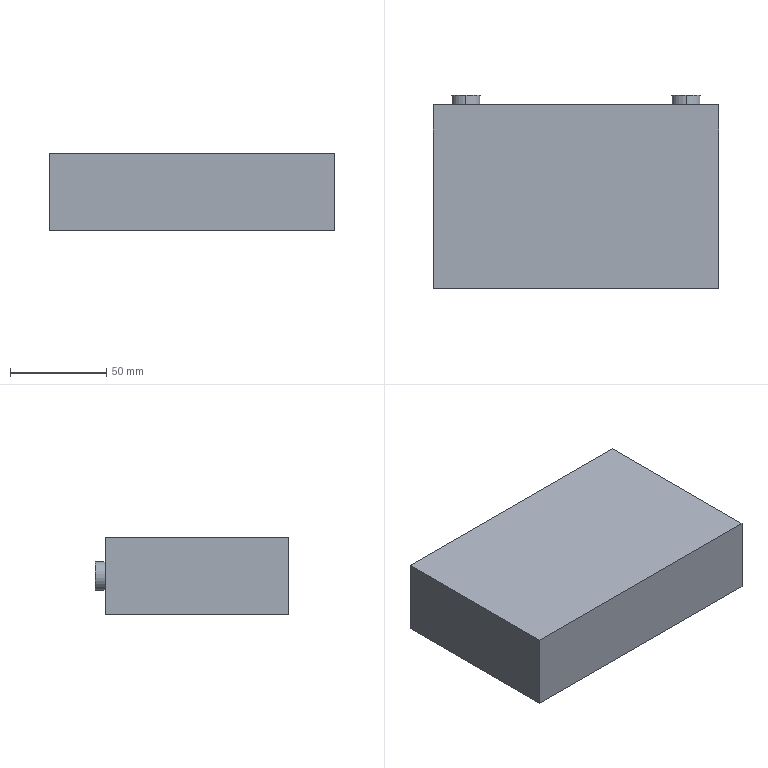Part | SolidWorks | features Extrusion 1, ICE 1 | 1 solid | 12 faces | box 148.9 x 100.6 x 40.2 mm | volume 574008 mm3 | plane 8 | cylinder 4 | commonest cylinder face diameters 15 x4
STEP:
#1=CARTESIAN_POINT('',(-57.3,100.6,7.5));
#2=VERTEX_POINT('',#1);
#3=CARTESIAN_POINT('',(-57.3,100.6,-7.5));
#4=VERTEX_POINT('',#3);
#5=CARTESIAN_POINT('',(-57.3,100.6,0.));
#6=DIRECTION('',(0.,1.,0.));
#7=DIRECTION('',(0.,0.,1.));
#8=AXIS2_PLACEMENT_3D('',#5,#6,#7);
#9=CIRCLE('',#8,7.5);
#10=EDGE_CURVE('',#2,#4,#9,.T.);
#11=ORIENTED_EDGE('',*,*,#10,.F.);
#12=CARTESIAN_POINT('',(-57.3,95.6,7.5));
#13=VERTEX_POINT('',#12);
#14=CARTESIAN_POINT('',(-57.3,100.6,7.5));
#15=DIRECTION('',(0.,-1.,0.));
#16=VECTOR('',#15,1000.);
#17=LINE('',#14,#16);
#18=EDGE_CURVE('',#2,#13,#17,.T.);
#19=ORIENTED_EDGE('',*,*,#18,.T.);
#20=CARTESIAN_POINT('',(-57.3,95.6,-7.5));
#21=VERTEX_POINT('',#20);
#22=CARTESIAN_POINT('',(-57.3,95.6,0.));
#23=DIRECTION('',(0.,1.,0.));
#24=DIRECTION('',(0.,0.,1.));
#25=AXIS2_PLACEMENT_3D('',#22,#23,#24);
#26=CIRCLE('',#25,7.5);
#27=EDGE_CURVE('',#13,#21,#26,.T.);
#28=ORIENTED_EDGE('',*,*,#27,.T.);
#29=CARTESIAN_POINT('',(-57.3,100.6,-7.5));
#30=DIRECTION('',(0.,-1.,0.));
#31=VECTOR('',#30,1000.);
#32=LINE('',#29,#31);
#33=EDGE_CURVE('',#4,#21,#32,.T.);
#34=ORIENTED_EDGE('',*,*,#33,.F.);
#35=EDGE_LOOP('',(#11,#19,#28,#34));
#36=FACE_OUTER_BOUND('',#35,.T.);
#37=CARTESIAN_POINT('',(-57.3,100.6,0.));
#38=DIRECTION('',(0.,-1.,0.));
#39=DIRECTION('',(0.,0.,-1.));
#40=AXIS2_PLACEMENT_3D('',#37,#38,#39);
#41=CYLINDRICAL_SURFACE('',#40,7.5);
#42=ADVANCED_FACE('',(#36),#41,.T.);
#43=CARTESIAN_POINT('',(57.3,100.6,7.5));
#44=VERTEX_POINT('',#43);
#45=CARTESIAN_POINT('',(57.3,100.6,-7.5));
#46=VERTEX_POINT('',#45);
#47=CARTESIAN_POINT('',(57.3,100.6,0.));
#48=DIRECTION('',(0.,1.,0.));
#49=DIRECTION('',(0.,0.,1.));
#50=AXIS2_PLACEMENT_3D('',#47,#48,#49);
#51=CIRCLE('',#50,7.5);
#52=EDGE_CURVE('',#44,#46,#51,.T.);
#53=ORIENTED_EDGE('',*,*,#52,.F.);
#54=CARTESIAN_POINT('',(57.3,95.6,7.5));
#55=VERTEX_POINT('',#54);
#56=CARTESIAN_POINT('',(57.3,100.6,7.5));
#57=DIRECTION('',(0.,-1.,0.));
#58=VECTOR('',#57,1000.);
#59=LINE('',#56,#58);
#60=EDGE_CURVE('',#44,#55,#59,.T.);
#61=ORIENTED_EDGE('',*,*,#60,.T.);
#62=CARTESIAN_POINT('',(57.3,95.6,-7.5));
#63=VERTEX_POINT('',#62);
#64=CARTESIAN_POINT('',(57.3,95.6,0.));
#65=DIRECTION('',(0.,1.,0.));
#66=DIRECTION('',(0.,0.,1.));
#67=AXIS2_PLACEMENT_3D('',#64,#65,#66);
#68=CIRCLE('',#67,7.5);
#69=EDGE_CURVE('',#55,#63,#68,.T.);
#70=ORIENTED_EDGE('',*,*,#69,.T.);
#71=CARTESIAN_POINT('',(57.3,100.6,-7.5));
#72=DIRECTION('',(0.,-1.,0.));
#73=VECTOR('',#72,1000.);
#74=LINE('',#71,#73);
#75=EDGE_CURVE('',#46,#63,#74,.T.);
#76=ORIENTED_EDGE('',*,*,#75,.F.);
#77=EDGE_LOOP('',(#53,#61,#70,#76));
#78=FACE_OUTER_BOUND('',#77,.T.);
#79=CARTESIAN_POINT('',(57.3,100.6,0.));
#80=DIRECTION('',(0.,-1.,0.));
#81=DIRECTION('',(0.,0.,-1.));
#82=AXIS2_PLACEMENT_3D('',#79,#80,#81);
#83=CYLINDRICAL_SURFACE('',#82,7.5);
#84=ADVANCED_FACE('',(#78),#83,.T.);
#85=CARTESIAN_POINT('',(57.3,95.6,0.));
#86=DIRECTION('',(0.,1.,0.));
#87=DIRECTION('',(0.,0.,1.));
#88=AXIS2_PLACEMENT_3D('',#85,#86,#87);
#89=CIRCLE('',#88,7.5);
#90=EDGE_CURVE('',#63,#55,#89,.T.);
#91=ORIENTED_EDGE('',*,*,#90,.F.);
#92=ORIENTED_EDGE('',*,*,#69,.F.);
#93=EDGE_LOOP('',(#91,#92));
#94=FACE_BOUND('',#93,.T.);
#95=CARTESIAN_POINT('',(74.45,95.6,20.1));
#96=VERTEX_POINT('',#95);
#97=CARTESIAN_POINT('',(74.45,95.6,-20.1));
#98=VERTEX_POINT('',#97);
#99=CARTESIAN_POINT('',(74.45,95.6,-20.1));
#100=DIRECTION('',(0.,0.,-1.));
#101=VECTOR('',#100,1000.);
#102=LINE('',#99,#101);
#103=EDGE_CURVE('',#96,#98,#102,.T.);
#104=ORIENTED_EDGE('',*,*,#103,.T.);
#105=CARTESIAN_POINT('',(-74.45,95.6,-20.1));
#106=VERTEX_POINT('',#105);
#107=CARTESIAN_POINT('',(-74.45,95.6,-20.1));
#108=DIRECTION('',(-1.,0.,0.));
#109=VECTOR('',#108,1000.);
#110=LINE('',#107,#109);
#111=EDGE_CURVE('',#98,#106,#110,.T.);
#112=ORIENTED_EDGE('',*,*,#111,.T.);
#113=CARTESIAN_POINT('',(-74.45,95.6,20.1));
#114=VERTEX_POINT('',#113);
#115=CARTESIAN_POINT('',(-74.45,95.6,-20.1));
#116=DIRECTION('',(0.,0.,1.));
#117=VECTOR('',#116,1000.);
#118=LINE('',#115,#117);
#119=EDGE_CURVE('',#106,#114,#118,.T.);
#120=ORIENTED_EDGE('',*,*,#119,.T.);
#121=CARTESIAN_POINT('',(-74.45,95.6,20.1));
#122=DIRECTION('',(1.,0.,0.));
#123=VECTOR('',#122,1000.);
#124=LINE('',#121,#123);
#125=EDGE_CURVE('',#114,#96,#124,.T.);
#126=ORIENTED_EDGE('',*,*,#125,.T.);
#127=EDGE_LOOP('',(#104,#112,#120,#126));
#128=FACE_OUTER_BOUND('',#127,.T.);
#129=CARTESIAN_POINT('',(-57.3,95.6,0.));
#130=DIRECTION('',(0.,1.,0.));
#131=DIRECTION('',(0.,0.,1.));
#132=AXIS2_PLACEMENT_3D('',#129,#130,#131);
#133=CIRCLE('',#132,7.5);
#134=EDGE_CURVE('',#21,#13,#133,.T.);
#135=ORIENTED_EDGE('',*,*,#134,.F.);
#136=ORIENTED_EDGE('',*,*,#27,.F.);
#137=EDGE_LOOP('',(#135,#136));
#138=FACE_BOUND('',#137,.T.);
#139=CARTESIAN_POINT('',(0.,95.6,0.));
#140=DIRECTION('',(0.,1.,0.));
#141=DIRECTION('',(0.,0.,1.));
#142=AXIS2_PLACEMENT_3D('',#139,#140,#141);
#143=PLANE('',#142);
#144=ADVANCED_FACE('',(#94,#128,#138),#143,.T.);
#145=CARTESIAN_POINT('',(74.45,0.,20.1));
#146=VERTEX_POINT('',#145);
#147=CARTESIAN_POINT('',(74.45,0.,-20.1));
#148=VERTEX_POINT('',#147);
#149=CARTESIAN_POINT('',(74.45,0.,-20.1));
#150=DIRECTION('',(0.,0.,-1.));
#151=VECTOR('',#150,1000.);
#152=LINE('',#149,#151);
#153=EDGE_CURVE('',#146,#148,#152,.T.);
#154=ORIENTED_EDGE('',*,*,#153,.T.);
#155=CARTESIAN_POINT('',(74.45,95.6,-20.1));
#156=DIRECTION('',(0.,-1.,0.));
#157=VECTOR('',#156,1000.);
#158=LINE('',#155,#157);
#159=EDGE_CURVE('',#98,#148,#158,.T.);
#160=ORIENTED_EDGE('',*,*,#159,.F.);
#161=ORIENTED_EDGE('',*,*,#103,.F.);
#162=CARTESIAN_POINT('',(74.45,95.6,20.1));
#163=DIRECTION('',(0.,-1.,0.));
#164=VECTOR('',#163,1000.);
#165=LINE('',#162,#164);
#166=EDGE_CURVE('',#96,#146,#165,.T.);
#167=ORIENTED_EDGE('',*,*,#166,.T.);
#168=EDGE_LOOP('',(#154,#160,#161,#167));
#169=FACE_OUTER_BOUND('',#168,.T.);
#170=CARTESIAN_POINT('',(74.45,95.6,-20.1));
#171=DIRECTION('',(-1.,0.,0.));
#172=DIRECTION('',(0.,0.,1.));
#173=AXIS2_PLACEMENT_3D('',#170,#171,#172);
#174=PLANE('',#173);
#175=ADVANCED_FACE('',(#169),#174,.F.);
#176=CARTESIAN_POINT('',(-74.45,0.,-20.1));
#177=VERTEX_POINT('',#176);
#178=CARTESIAN_POINT('',(-74.45,0.,-20.1));
#179=DIRECTION('',(-1.,0.,0.));
#180=VECTOR('',#179,1000.);
#181=LINE('',#178,#180);
#182=EDGE_CURVE('',#148,#177,#181,.T.);
#183=ORIENTED_EDGE('',*,*,#182,.T.);
#184=CARTESIAN_POINT('',(-74.45,95.6,-20.1));
#185=DIRECTION('',(0.,-1.,0.));
#186=VECTOR('',#185,1000.);
#187=LINE('',#184,#186);
#188=EDGE_CURVE('',#106,#177,#187,.T.);
#189=ORIENTED_EDGE('',*,*,#188,.F.);
#190=ORIENTED_EDGE('',*,*,#111,.F.);
#191=ORIENTED_EDGE('',*,*,#159,.T.);
#192=EDGE_LOOP('',(#183,#189,#190,#191));
#193=FACE_OUTER_BOUND('',#192,.T.);
#194=CARTESIAN_POINT('',(-74.45,95.6,-20.1));
#195=DIRECTION('',(0.,0.,1.));
#196=DIRECTION('',(1.,0.,0.));
#197=AXIS2_PLACEMENT_3D('',#194,#195,#196);
#198=PLANE('',#197);
#199=ADVANCED_FACE('',(#193),#198,.F.);
#200=CARTESIAN_POINT('',(-74.45,0.,20.1));
#201=VERTEX_POINT('',#200);
#202=CARTESIAN_POINT('',(-74.45,0.,-20.1));
#203=DIRECTION('',(0.,0.,1.));
#204=VECTOR('',#203,1000.);
#205=LINE('',#202,#204);
#206=EDGE_CURVE('',#177,#201,#205,.T.);
#207=ORIENTED_EDGE('',*,*,#206,.T.);
#208=CARTESIAN_POINT('',(-74.45,95.6,20.1));
#209=DIRECTION('',(0.,-1.,0.));
#210=VECTOR('',#209,1000.);
#211=LINE('',#208,#210);
#212=EDGE_CURVE('',#114,#201,#211,.T.);
#213=ORIENTED_EDGE('',*,*,#212,.F.);
#214=ORIENTED_EDGE('',*,*,#119,.F.);
#215=ORIENTED_EDGE('',*,*,#188,.T.);
#216=EDGE_LOOP('',(#207,#213,#214,#215));
#217=FACE_OUTER_BOUND('',#216,.T.);
#218=CARTESIAN_POINT('',(-74.45,95.6,-20.1));
#219=DIRECTION('',(1.,0.,0.));
#220=DIRECTION('',(0.,0.,-1.));
#221=AXIS2_PLACEMENT_3D('',#218,#219,#220);
#222=PLANE('',#221);
#223=ADVANCED_FACE('',(#217),#222,.F.);
#224=CARTESIAN_POINT('',(-74.45,0.,20.1));
#225=DIRECTION('',(1.,0.,0.));
#226=VECTOR('',#225,1000.);
#227=LINE('',#224,#226);
#228=EDGE_CURVE('',#201,#146,#227,.T.);
#229=ORIENTED_EDGE('',*,*,#228,.T.);
#230=ORIENTED_EDGE('',*,*,#166,.F.);
#231=ORIENTED_EDGE('',*,*,#125,.F.);
#232=ORIENTED_EDGE('',*,*,#212,.T.);
#233=EDGE_LOOP('',(#229,#230,#231,#232));
#234=FACE_OUTER_BOUND('',#233,.T.);
#235=CARTESIAN_POINT('',(-74.45,95.6,20.1));
#236=DIRECTION('',(0.,0.,-1.));
#237=DIRECTION('',(-1.,0.,0.));
#238=AXIS2_PLACEMENT_3D('',#235,#236,#237);
#239=PLANE('',#238);
#240=ADVANCED_FACE('',(#234),#239,.F.);
#241=ORIENTED_EDGE('',*,*,#153,.F.);
#242=ORIENTED_EDGE('',*,*,#228,.F.);
#243=ORIENTED_EDGE('',*,*,#206,.F.);
#244=ORIENTED_EDGE('',*,*,#182,.F.);
#245=EDGE_LOOP('',(#241,#242,#243,#244));
#246=FACE_OUTER_BOUND('',#245,.T.);
#247=CARTESIAN_POINT('',(0.,0.,0.));
#248=DIRECTION('',(0.,1.,0.));
#249=DIRECTION('',(0.,0.,1.));
#250=AXIS2_PLACEMENT_3D('',#247,#248,#249);
#251=PLANE('',#250);
#252=ADVANCED_FACE('',(#246),#251,.F.);
#253=ORIENTED_EDGE('',*,*,#60,.F.);
#254=CARTESIAN_POINT('',(57.3,100.6,0.));
#255=DIRECTION('',(0.,1.,0.));
#256=DIRECTION('',(0.,0.,1.));
#257=AXIS2_PLACEMENT_3D('',#254,#255,#256);
#258=CIRCLE('',#257,7.5);
#259=EDGE_CURVE('',#46,#44,#258,.T.);
#260=ORIENTED_EDGE('',*,*,#259,.F.);
#261=ORIENTED_EDGE('',*,*,#75,.T.);
#262=ORIENTED_EDGE('',*,*,#90,.T.);
#263=EDGE_LOOP('',(#253,#260,#261,#262));
#264=FACE_OUTER_BOUND('',#263,.T.);
#265=CARTESIAN_POINT('',(57.3,100.6,0.));
#266=DIRECTION('',(0.,-1.,0.));
#267=DIRECTION('',(0.,0.,-1.));
#268=AXIS2_PLACEMENT_3D('',#265,#266,#267);
#269=CYLINDRICAL_SURFACE('',#268,7.5);
#270=ADVANCED_FACE('',(#264),#269,.T.);
#271=ORIENTED_EDGE('',*,*,#259,.T.);
#272=ORIENTED_EDGE('',*,*,#52,.T.);
#273=EDGE_LOOP('',(#271,#272));
#274=FACE_OUTER_BOUND('',#273,.T.);
#275=CARTESIAN_POINT('',(57.3,100.6,0.));
#276=DIRECTION('',(0.,1.,0.));
#277=DIRECTION('',(0.,0.,1.));
#278=AXIS2_PLACEMENT_3D('',#275,#276,#277);
#279=PLANE('',#278);
#280=ADVANCED_FACE('',(#274),#279,.T.);
#281=ORIENTED_EDGE('',*,*,#18,.F.);
#282=CARTESIAN_POINT('',(-57.3,100.6,0.));
#283=DIRECTION('',(0.,1.,0.));
#284=DIRECTION('',(0.,0.,1.));
#285=AXIS2_PLACEMENT_3D('',#282,#283,#284);
#286=CIRCLE('',#285,7.5);
#287=EDGE_CURVE('',#4,#2,#286,.T.);
#288=ORIENTED_EDGE('',*,*,#287,.F.);
#289=ORIENTED_EDGE('',*,*,#33,.T.);
#290=ORIENTED_EDGE('',*,*,#134,.T.);
#291=EDGE_LOOP('',(#281,#288,#289,#290));
#292=FACE_OUTER_BOUND('',#291,.T.);
#293=CARTESIAN_POINT('',(-57.3,100.6,0.));
#294=DIRECTION('',(0.,-1.,0.));
#295=DIRECTION('',(0.,0.,-1.));
#296=AXIS2_PLACEMENT_3D('',#293,#294,#295);
#297=CYLINDRICAL_SURFACE('',#296,7.5);
#298=ADVANCED_FACE('',(#292),#297,.T.);
#299=ORIENTED_EDGE('',*,*,#287,.T.);
#300=ORIENTED_EDGE('',*,*,#10,.T.);
#301=EDGE_LOOP('',(#299,#300));
#302=FACE_OUTER_BOUND('',#301,.T.);
#303=CARTESIAN_POINT('',(-57.3,100.6,0.));
#304=DIRECTION('',(0.,1.,0.));
#305=DIRECTION('',(0.,0.,1.));
#306=AXIS2_PLACEMENT_3D('',#303,#304,#305);
#307=PLANE('',#306);
#308=ADVANCED_FACE('',(#302),#307,.T.);
#309=CLOSED_SHELL('',(#42,#84,#144,#175,#199,#223,#240,#252,#270,#280,#298,#308));
#310=MANIFOLD_SOLID_BREP('',#309);
#311=CARTESIAN_POINT('',(0.,0.,0.));
#312=DIRECTION('',(0.,0.,1.));
#313=DIRECTION('',(1.,0.,0.));
#314=AXIS2_PLACEMENT_3D('',#311,#312,#313);
#315=(LENGTH_UNIT()NAMED_UNIT(*)SI_UNIT(.MILLI.,.METRE.));
#316=UNCERTAINTY_MEASURE_WITH_UNIT(LENGTH_MEASURE(0.00001),#315,'','');
#317=(NAMED_UNIT(*)PLANE_ANGLE_UNIT()SI_UNIT($,.RADIAN.));
#318=(NAMED_UNIT(*)SI_UNIT($,.STERADIAN.)SOLID_ANGLE_UNIT());
#319=(GEOMETRIC_REPRESENTATION_CONTEXT(3)GLOBAL_UNCERTAINTY_ASSIGNED_CONTEXT((#316))GLOBAL_UNIT_ASSIGNED_CONTEXT((#315,#317,#318))REPRESENTATION_CONTEXT('',''));
#320=ADVANCED_BREP_SHAPE_REPRESENTATION('',(#310,#314),#319);